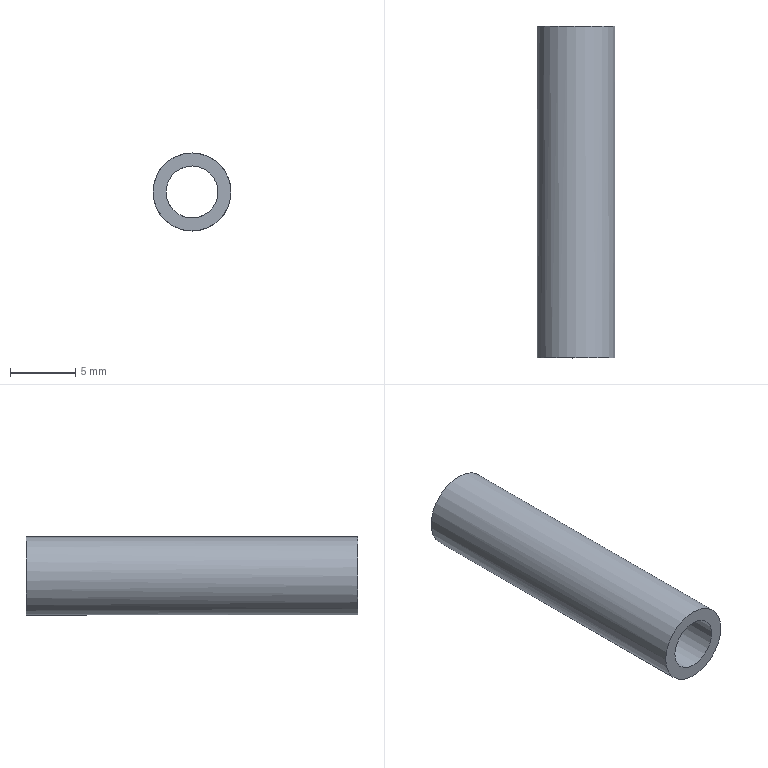Part | NX | features solid 2 | 1 solid | 4 faces | box 6 x 25.512 x 6 mm | volume 400.744 mm3 | cylinder 2 | plane 2 | commonest cylinder face diameters 4 x1 6 x1
STEP:
#1=CARTESIAN_POINT('',(271.,-17.125,347.));
#2=VERTEX_POINT('',#1);
#3=CARTESIAN_POINT('',(273.,-17.125,347.));
#4=DIRECTION('',(0.,1.,0.));
#5=DIRECTION('',(-1.,0.,0.));
#6=AXIS2_PLACEMENT_3D('',#3,#4,#5);
#7=CIRCLE('',#6,2.);
#8=EDGE_CURVE('',#2,#2,#7,.T.);
#9=ORIENTED_EDGE('',*,*,#8,.F.);
#10=EDGE_LOOP('',(#9));
#11=FACE_BOUND('',#10,.T.);
#12=CARTESIAN_POINT('',(273.,8.387,349.));
#13=VERTEX_POINT('',#12);
#14=CARTESIAN_POINT('',(273.,8.387,347.));
#15=DIRECTION('',(0.,1.,0.));
#16=DIRECTION('',(0.,0.,1.));
#17=AXIS2_PLACEMENT_3D('',#14,#15,#16);
#18=CIRCLE('',#17,2.);
#19=EDGE_CURVE('',#13,#13,#18,.T.);
#20=ORIENTED_EDGE('',*,*,#19,.T.);
#21=EDGE_LOOP('',(#20));
#22=FACE_BOUND('',#21,.T.);
#23=CARTESIAN_POINT('',(273.,53.824,347.));
#24=DIRECTION('',(0.,-1.,0.));
#25=DIRECTION('',(1.,0.,0.));
#26=AXIS2_PLACEMENT_3D('',#23,#24,#25);
#27=CYLINDRICAL_SURFACE('',#26,2.);
#28=ADVANCED_FACE('',(#11,#22),#27,.F.);
#29=ORIENTED_EDGE('',*,*,#19,.F.);
#30=EDGE_LOOP('',(#29));
#31=FACE_BOUND('',#30,.T.);
#32=CARTESIAN_POINT('',(273.,8.387,350.));
#33=VERTEX_POINT('',#32);
#34=CARTESIAN_POINT('',(273.,8.387,347.));
#35=DIRECTION('',(0.,1.,0.));
#36=DIRECTION('',(0.,0.,1.));
#37=AXIS2_PLACEMENT_3D('',#34,#35,#36);
#38=CIRCLE('',#37,3.);
#39=EDGE_CURVE('',#33,#33,#38,.T.);
#40=ORIENTED_EDGE('',*,*,#39,.T.);
#41=EDGE_LOOP('',(#40));
#42=FACE_BOUND('',#41,.T.);
#43=CARTESIAN_POINT('',(377.131,8.387,203.));
#44=DIRECTION('',(0.,1.,0.));
#45=DIRECTION('',(0.,0.,1.));
#46=AXIS2_PLACEMENT_3D('',#43,#44,#45);
#47=PLANE('',#46);
#48=ADVANCED_FACE('',(#31,#42),#47,.T.);
#49=CARTESIAN_POINT('',(270.,-17.125,347.));
#50=VERTEX_POINT('',#49);
#51=CARTESIAN_POINT('',(273.,-17.125,347.));
#52=DIRECTION('',(0.,1.,0.));
#53=DIRECTION('',(-1.,0.,0.));
#54=AXIS2_PLACEMENT_3D('',#51,#52,#53);
#55=CIRCLE('',#54,3.);
#56=EDGE_CURVE('',#50,#50,#55,.T.);
#57=ORIENTED_EDGE('',*,*,#56,.T.);
#58=EDGE_LOOP('',(#57));
#59=FACE_BOUND('',#58,.T.);
#60=ORIENTED_EDGE('',*,*,#39,.F.);
#61=EDGE_LOOP('',(#60));
#62=FACE_BOUND('',#61,.T.);
#63=CARTESIAN_POINT('',(273.,53.824,347.));
#64=DIRECTION('',(0.,-1.,0.));
#65=DIRECTION('',(1.,0.,0.));
#66=AXIS2_PLACEMENT_3D('',#63,#64,#65);
#67=CYLINDRICAL_SURFACE('',#66,3.);
#68=ADVANCED_FACE('',(#59,#62),#67,.T.);
#69=ORIENTED_EDGE('',*,*,#8,.T.);
#70=EDGE_LOOP('',(#69));
#71=FACE_BOUND('',#70,.T.);
#72=ORIENTED_EDGE('',*,*,#56,.F.);
#73=EDGE_LOOP('',(#72));
#74=FACE_BOUND('',#73,.T.);
#75=CARTESIAN_POINT('',(397.83,-17.125,185.));
#76=DIRECTION('',(0.,1.,0.));
#77=DIRECTION('',(-1.,0.,0.));
#78=AXIS2_PLACEMENT_3D('',#75,#76,#77);
#79=PLANE('',#78);
#80=ADVANCED_FACE('',(#71,#74),#79,.F.);
#81=CLOSED_SHELL('',(#28,#48,#68,#80));
#82=MANIFOLD_SOLID_BREP('',#81);
#83=(LENGTH_UNIT()NAMED_UNIT(*)SI_UNIT(.MILLI.,.METRE.));
#84=UNCERTAINTY_MEASURE_WITH_UNIT(LENGTH_MEASURE(0.00001),#83,'','');
#85=(NAMED_UNIT(*)PLANE_ANGLE_UNIT()SI_UNIT($,.RADIAN.));
#86=(NAMED_UNIT(*)SI_UNIT($,.STERADIAN.)SOLID_ANGLE_UNIT());
#87=(GEOMETRIC_REPRESENTATION_CONTEXT(3)GLOBAL_UNCERTAINTY_ASSIGNED_CONTEXT((#84))GLOBAL_UNIT_ASSIGNED_CONTEXT((#83,#85,#86))REPRESENTATION_CONTEXT('',''));
#88=ADVANCED_BREP_SHAPE_REPRESENTATION('',(#82),#87);